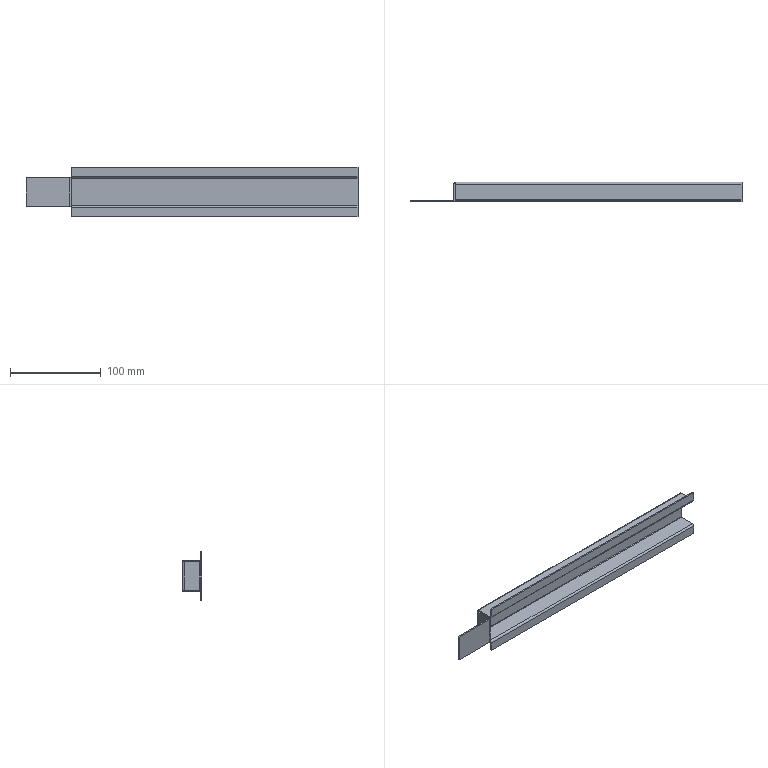Part | STEP file | 750078364 | 1 solid | 38 faces | box 366.5 x 21.5 x 55 mm | volume 47287 mm3 | plane 26 | cylinder 12 | commonest cylinder face diameters 1 x6 4 x6
STEP:
#1=CARTESIAN_POINT('',(-157.,20.,15.));
#2=VERTEX_POINT('',#1);
#3=CARTESIAN_POINT('',(-157.,20.,-15.));
#4=VERTEX_POINT('',#3);
#5=CARTESIAN_POINT('',(-157.,20.,15.));
#6=DIRECTION('',(0.,0.,-1.));
#7=VECTOR('',#6,1000.);
#8=LINE('',#5,#7);
#9=EDGE_CURVE('',#2,#4,#8,.T.);
#10=ORIENTED_EDGE('',*,*,#9,.F.);
#11=CARTESIAN_POINT('',(159.,20.,15.));
#12=VERTEX_POINT('',#11);
#13=CARTESIAN_POINT('',(159.,20.,15.));
#14=DIRECTION('',(-1.,0.,0.));
#15=VECTOR('',#14,1000.);
#16=LINE('',#13,#15);
#17=EDGE_CURVE('',#12,#2,#16,.T.);
#18=ORIENTED_EDGE('',*,*,#17,.F.);
#19=CARTESIAN_POINT('',(159.,20.,-15.));
#20=VERTEX_POINT('',#19);
#21=CARTESIAN_POINT('',(159.,20.,15.));
#22=DIRECTION('',(0.,0.,1.));
#23=VECTOR('',#22,1000.);
#24=LINE('',#21,#23);
#25=EDGE_CURVE('',#20,#12,#24,.T.);
#26=ORIENTED_EDGE('',*,*,#25,.F.);
#27=CARTESIAN_POINT('',(159.,20.,-15.));
#28=DIRECTION('',(1.,0.,0.));
#29=VECTOR('',#28,1000.);
#30=LINE('',#27,#29);
#31=EDGE_CURVE('',#4,#20,#30,.T.);
#32=ORIENTED_EDGE('',*,*,#31,.F.);
#33=EDGE_LOOP('',(#10,#18,#26,#32));
#34=FACE_OUTER_BOUND('',#33,.T.);
#35=CARTESIAN_POINT('',(159.,20.,15.));
#36=DIRECTION('',(0.,-1.,0.));
#37=DIRECTION('',(1.,0.,0.));
#38=AXIS2_PLACEMENT_3D('',#35,#36,#37);
#39=PLANE('',#38);
#40=ADVANCED_FACE('',(#34),#39,.F.);
#41=CARTESIAN_POINT('',(159.,18.,-17.));
#42=VERTEX_POINT('',#41);
#43=CARTESIAN_POINT('',(-157.498,18.,-17.));
#44=VERTEX_POINT('',#43);
#45=CARTESIAN_POINT('',(-157.,18.,-17.));
#46=DIRECTION('',(-1.,0.,0.));
#47=VECTOR('',#46,1000.);
#48=LINE('',#45,#47);
#49=EDGE_CURVE('',#42,#44,#48,.T.);
#50=ORIENTED_EDGE('',*,*,#49,.T.);
#51=CARTESIAN_POINT('',(-157.498,19.936,-15.5));
#52=VERTEX_POINT('',#51);
#53=CARTESIAN_POINT('',(-157.498,18.,-15.));
#54=DIRECTION('',(1.,0.,0.));
#55=DIRECTION('',(0.,1.,0.));
#56=AXIS2_PLACEMENT_3D('',#53,#54,#55);
#57=CIRCLE('',#56,2.);
#58=EDGE_CURVE('',#44,#52,#57,.T.);
#59=ORIENTED_EDGE('',*,*,#58,.T.);
#60=CARTESIAN_POINT('',(-157.,20.,-15.));
#61=CARTESIAN_POINT('',(-157.168,20.,-15.169));
#62=CARTESIAN_POINT('',(-157.335,19.979,-15.336));
#63=CARTESIAN_POINT('',(-157.498,19.936,-15.5));
#64=(BOUNDED_CURVE()B_SPLINE_CURVE(3,(#60,#61,#62,#63),.UNSPECIFIED.,.F.,.F.)B_SPLINE_CURVE_WITH_KNOTS((4,4),(1.571,1.823),.UNSPECIFIED.)CURVE()GEOMETRIC_REPRESENTATION_ITEM()RATIONAL_B_SPLINE_CURVE((1.,0.9947,0.9947,1.))REPRESENTATION_ITEM(''));
#65=EDGE_CURVE('',#4,#52,#64,.T.);
#66=ORIENTED_EDGE('',*,*,#65,.F.);
#67=ORIENTED_EDGE('',*,*,#31,.T.);
#68=CARTESIAN_POINT('',(159.,18.,-15.));
#69=DIRECTION('',(-1.,0.,0.));
#70=DIRECTION('',(0.,1.,0.));
#71=AXIS2_PLACEMENT_3D('',#68,#69,#70);
#72=CIRCLE('',#71,2.);
#73=EDGE_CURVE('',#20,#42,#72,.T.);
#74=ORIENTED_EDGE('',*,*,#73,.T.);
#75=EDGE_LOOP('',(#50,#59,#66,#67,#74));
#76=FACE_OUTER_BOUND('',#75,.T.);
#77=CARTESIAN_POINT('',(-157.,18.,-15.));
#78=DIRECTION('',(1.,0.,0.));
#79=DIRECTION('',(0.,1.,0.));
#80=AXIS2_PLACEMENT_3D('',#77,#78,#79);
#81=CYLINDRICAL_SURFACE('',#80,2.);
#82=ADVANCED_FACE('',(#76),#81,.T.);
#83=CARTESIAN_POINT('',(-159.,18.,-15.498));
#84=VERTEX_POINT('',#83);
#85=CARTESIAN_POINT('',(-159.,18.,15.498));
#86=VERTEX_POINT('',#85);
#87=CARTESIAN_POINT('',(-159.,18.,15.));
#88=DIRECTION('',(0.,0.,1.));
#89=VECTOR('',#88,1000.);
#90=LINE('',#87,#89);
#91=EDGE_CURVE('',#84,#86,#90,.T.);
#92=ORIENTED_EDGE('',*,*,#91,.T.);
#93=CARTESIAN_POINT('',(-157.5,19.936,15.498));
#94=VERTEX_POINT('',#93);
#95=CARTESIAN_POINT('',(-157.,18.,15.498));
#96=DIRECTION('',(0.,0.,-1.));
#97=DIRECTION('',(-1.,0.,0.));
#98=AXIS2_PLACEMENT_3D('',#95,#96,#97);
#99=CIRCLE('',#98,2.);
#100=EDGE_CURVE('',#86,#94,#99,.T.);
#101=ORIENTED_EDGE('',*,*,#100,.T.);
#102=CARTESIAN_POINT('',(-157.,20.,15.));
#103=CARTESIAN_POINT('',(-157.169,20.,15.168));
#104=CARTESIAN_POINT('',(-157.336,19.979,15.335));
#105=CARTESIAN_POINT('',(-157.5,19.936,15.498));
#106=(BOUNDED_CURVE()B_SPLINE_CURVE(3,(#102,#103,#104,#105),.UNSPECIFIED.,.F.,.F.)B_SPLINE_CURVE_WITH_KNOTS((4,4),(1.571,1.823),.UNSPECIFIED.)CURVE()GEOMETRIC_REPRESENTATION_ITEM()RATIONAL_B_SPLINE_CURVE((1.,0.9947,0.9947,1.))REPRESENTATION_ITEM(''));
#107=EDGE_CURVE('',#2,#94,#106,.T.);
#108=ORIENTED_EDGE('',*,*,#107,.F.);
#109=ORIENTED_EDGE('',*,*,#9,.T.);
#110=CARTESIAN_POINT('',(-157.5,19.936,-15.498));
#111=VERTEX_POINT('',#110);
#112=CARTESIAN_POINT('',(-157.,20.,-15.));
#113=CARTESIAN_POINT('',(-157.169,20.,-15.168));
#114=CARTESIAN_POINT('',(-157.336,19.979,-15.335));
#115=CARTESIAN_POINT('',(-157.5,19.936,-15.498));
#116=(BOUNDED_CURVE()B_SPLINE_CURVE(3,(#112,#113,#114,#115),.UNSPECIFIED.,.F.,.F.)B_SPLINE_CURVE_WITH_KNOTS((4,4),(4.712,4.965),.UNSPECIFIED.)CURVE()GEOMETRIC_REPRESENTATION_ITEM()RATIONAL_B_SPLINE_CURVE((1.,0.9947,0.9947,1.))REPRESENTATION_ITEM(''));
#117=EDGE_CURVE('',#4,#111,#116,.T.);
#118=ORIENTED_EDGE('',*,*,#117,.T.);
#119=CARTESIAN_POINT('',(-157.,18.,-15.498));
#120=DIRECTION('',(0.,0.,1.));
#121=DIRECTION('',(-1.,0.,0.));
#122=AXIS2_PLACEMENT_3D('',#119,#120,#121);
#123=CIRCLE('',#122,2.);
#124=EDGE_CURVE('',#111,#84,#123,.T.);
#125=ORIENTED_EDGE('',*,*,#124,.T.);
#126=EDGE_LOOP('',(#92,#101,#108,#109,#118,#125));
#127=FACE_OUTER_BOUND('',#126,.T.);
#128=CARTESIAN_POINT('',(-157.,18.,15.));
#129=DIRECTION('',(0.,0.,-1.));
#130=DIRECTION('',(-1.,0.,0.));
#131=AXIS2_PLACEMENT_3D('',#128,#129,#130);
#132=CYLINDRICAL_SURFACE('',#131,2.);
#133=ADVANCED_FACE('',(#127),#132,.T.);
#134=CARTESIAN_POINT('',(-157.498,18.,17.));
#135=VERTEX_POINT('',#134);
#136=CARTESIAN_POINT('',(159.,18.,17.));
#137=VERTEX_POINT('',#136);
#138=CARTESIAN_POINT('',(159.,18.,17.));
#139=DIRECTION('',(1.,0.,0.));
#140=VECTOR('',#139,1000.);
#141=LINE('',#138,#140);
#142=EDGE_CURVE('',#135,#137,#141,.T.);
#143=ORIENTED_EDGE('',*,*,#142,.T.);
#144=CARTESIAN_POINT('',(159.,18.,15.));
#145=DIRECTION('',(-1.,0.,0.));
#146=DIRECTION('',(0.,-1.,0.));
#147=AXIS2_PLACEMENT_3D('',#144,#145,#146);
#148=CIRCLE('',#147,2.);
#149=EDGE_CURVE('',#137,#12,#148,.T.);
#150=ORIENTED_EDGE('',*,*,#149,.T.);
#151=ORIENTED_EDGE('',*,*,#17,.T.);
#152=CARTESIAN_POINT('',(-157.498,19.936,15.5));
#153=VERTEX_POINT('',#152);
#154=CARTESIAN_POINT('',(-157.,20.,15.));
#155=CARTESIAN_POINT('',(-157.168,20.,15.169));
#156=CARTESIAN_POINT('',(-157.335,19.979,15.336));
#157=CARTESIAN_POINT('',(-157.498,19.936,15.5));
#158=(BOUNDED_CURVE()B_SPLINE_CURVE(3,(#154,#155,#156,#157),.UNSPECIFIED.,.F.,.F.)B_SPLINE_CURVE_WITH_KNOTS((4,4),(4.712,4.965),.UNSPECIFIED.)CURVE()GEOMETRIC_REPRESENTATION_ITEM()RATIONAL_B_SPLINE_CURVE((1.,0.9947,0.9947,1.))REPRESENTATION_ITEM(''));
#159=EDGE_CURVE('',#2,#153,#158,.T.);
#160=ORIENTED_EDGE('',*,*,#159,.T.);
#161=CARTESIAN_POINT('',(-157.498,18.,15.));
#162=DIRECTION('',(1.,0.,0.));
#163=DIRECTION('',(0.,-1.,0.));
#164=AXIS2_PLACEMENT_3D('',#161,#162,#163);
#165=CIRCLE('',#164,2.);
#166=EDGE_CURVE('',#153,#135,#165,.T.);
#167=ORIENTED_EDGE('',*,*,#166,.T.);
#168=EDGE_LOOP('',(#143,#150,#151,#160,#167));
#169=FACE_OUTER_BOUND('',#168,.T.);
#170=CARTESIAN_POINT('',(159.,18.,15.));
#171=DIRECTION('',(-1.,0.,0.));
#172=DIRECTION('',(0.,-1.,0.));
#173=AXIS2_PLACEMENT_3D('',#170,#171,#172);
#174=CYLINDRICAL_SURFACE('',#173,2.);
#175=ADVANCED_FACE('',(#169),#174,.T.);
#176=ORIENTED_EDGE('',*,*,#25,.T.);
#177=ORIENTED_EDGE('',*,*,#149,.F.);
#178=CARTESIAN_POINT('',(159.,0.5,17.));
#179=VERTEX_POINT('',#178);
#180=CARTESIAN_POINT('',(159.,20.,17.));
#181=DIRECTION('',(0.,1.,0.));
#182=VECTOR('',#181,1000.);
#183=LINE('',#180,#182);
#184=EDGE_CURVE('',#179,#137,#183,.T.);
#185=ORIENTED_EDGE('',*,*,#184,.F.);
#186=CARTESIAN_POINT('',(159.,0.,17.5));
#187=VERTEX_POINT('',#186);
#188=CARTESIAN_POINT('',(159.,0.5,17.5));
#189=DIRECTION('',(-1.,0.,0.));
#190=DIRECTION('',(0.,1.,0.));
#191=AXIS2_PLACEMENT_3D('',#188,#189,#190);
#192=CIRCLE('',#191,0.5);
#193=EDGE_CURVE('',#179,#187,#192,.T.);
#194=ORIENTED_EDGE('',*,*,#193,.T.);
#195=CARTESIAN_POINT('',(159.,0.,27.5));
#196=VERTEX_POINT('',#195);
#197=CARTESIAN_POINT('',(159.,0.,15.));
#198=DIRECTION('',(0.,0.,-1.));
#199=VECTOR('',#198,1000.);
#200=LINE('',#197,#199);
#201=EDGE_CURVE('',#196,#187,#200,.T.);
#202=ORIENTED_EDGE('',*,*,#201,.F.);
#203=CARTESIAN_POINT('',(159.,-1.5,27.5));
#204=VERTEX_POINT('',#203);
#205=CARTESIAN_POINT('',(159.,0.,27.5));
#206=DIRECTION('',(0.,1.,0.));
#207=VECTOR('',#206,1000.);
#208=LINE('',#205,#207);
#209=EDGE_CURVE('',#204,#196,#208,.T.);
#210=ORIENTED_EDGE('',*,*,#209,.F.);
#211=CARTESIAN_POINT('',(159.,-1.5,17.5));
#212=VERTEX_POINT('',#211);
#213=CARTESIAN_POINT('',(159.,-1.5,15.));
#214=DIRECTION('',(0.,0.,1.));
#215=VECTOR('',#214,1000.);
#216=LINE('',#213,#215);
#217=EDGE_CURVE('',#212,#204,#216,.T.);
#218=ORIENTED_EDGE('',*,*,#217,.F.);
#219=CARTESIAN_POINT('',(159.,0.5,15.5));
#220=VERTEX_POINT('',#219);
#221=CARTESIAN_POINT('',(159.,0.5,17.5));
#222=DIRECTION('',(-1.,0.,0.));
#223=DIRECTION('',(0.,1.,0.));
#224=AXIS2_PLACEMENT_3D('',#221,#222,#223);
#225=CIRCLE('',#224,2.);
#226=EDGE_CURVE('',#220,#212,#225,.T.);
#227=ORIENTED_EDGE('',*,*,#226,.F.);
#228=CARTESIAN_POINT('',(159.,18.,15.5));
#229=VERTEX_POINT('',#228);
#230=CARTESIAN_POINT('',(159.,20.,15.5));
#231=DIRECTION('',(0.,-1.,0.));
#232=VECTOR('',#231,1000.);
#233=LINE('',#230,#232);
#234=EDGE_CURVE('',#229,#220,#233,.T.);
#235=ORIENTED_EDGE('',*,*,#234,.F.);
#236=CARTESIAN_POINT('',(159.,18.5,15.));
#237=VERTEX_POINT('',#236);
#238=CARTESIAN_POINT('',(159.,18.,15.));
#239=DIRECTION('',(-1.,0.,0.));
#240=DIRECTION('',(0.,-1.,0.));
#241=AXIS2_PLACEMENT_3D('',#238,#239,#240);
#242=CIRCLE('',#241,0.5);
#243=EDGE_CURVE('',#229,#237,#242,.T.);
#244=ORIENTED_EDGE('',*,*,#243,.T.);
#245=CARTESIAN_POINT('',(159.,18.5,-15.));
#246=VERTEX_POINT('',#245);
#247=CARTESIAN_POINT('',(159.,18.5,15.));
#248=DIRECTION('',(0.,0.,1.));
#249=VECTOR('',#248,1000.);
#250=LINE('',#247,#249);
#251=EDGE_CURVE('',#246,#237,#250,.T.);
#252=ORIENTED_EDGE('',*,*,#251,.F.);
#253=CARTESIAN_POINT('',(159.,18.,-15.5));
#254=VERTEX_POINT('',#253);
#255=CARTESIAN_POINT('',(159.,18.,-15.));
#256=DIRECTION('',(-1.,0.,0.));
#257=DIRECTION('',(0.,1.,0.));
#258=AXIS2_PLACEMENT_3D('',#255,#256,#257);
#259=CIRCLE('',#258,0.5);
#260=EDGE_CURVE('',#246,#254,#259,.T.);
#261=ORIENTED_EDGE('',*,*,#260,.T.);
#262=CARTESIAN_POINT('',(159.,0.5,-15.5));
#263=VERTEX_POINT('',#262);
#264=CARTESIAN_POINT('',(159.,20.,-15.5));
#265=DIRECTION('',(0.,1.,0.));
#266=VECTOR('',#265,1000.);
#267=LINE('',#264,#266);
#268=EDGE_CURVE('',#263,#254,#267,.T.);
#269=ORIENTED_EDGE('',*,*,#268,.F.);
#270=CARTESIAN_POINT('',(159.,-1.5,-17.5));
#271=VERTEX_POINT('',#270);
#272=CARTESIAN_POINT('',(159.,0.5,-17.5));
#273=DIRECTION('',(-1.,0.,0.));
#274=DIRECTION('',(0.,-1.,0.));
#275=AXIS2_PLACEMENT_3D('',#272,#273,#274);
#276=CIRCLE('',#275,2.);
#277=EDGE_CURVE('',#271,#263,#276,.T.);
#278=ORIENTED_EDGE('',*,*,#277,.F.);
#279=CARTESIAN_POINT('',(159.,-1.5,-27.5));
#280=VERTEX_POINT('',#279);
#281=CARTESIAN_POINT('',(159.,-1.5,15.));
#282=DIRECTION('',(0.,0.,1.));
#283=VECTOR('',#282,1000.);
#284=LINE('',#281,#283);
#285=EDGE_CURVE('',#280,#271,#284,.T.);
#286=ORIENTED_EDGE('',*,*,#285,.F.);
#287=CARTESIAN_POINT('',(159.,0.,-27.5));
#288=VERTEX_POINT('',#287);
#289=CARTESIAN_POINT('',(159.,0.,-27.5));
#290=DIRECTION('',(0.,-1.,0.));
#291=VECTOR('',#290,1000.);
#292=LINE('',#289,#291);
#293=EDGE_CURVE('',#288,#280,#292,.T.);
#294=ORIENTED_EDGE('',*,*,#293,.F.);
#295=CARTESIAN_POINT('',(159.,0.,-17.5));
#296=VERTEX_POINT('',#295);
#297=CARTESIAN_POINT('',(159.,0.,15.));
#298=DIRECTION('',(0.,0.,-1.));
#299=VECTOR('',#298,1000.);
#300=LINE('',#297,#299);
#301=EDGE_CURVE('',#296,#288,#300,.T.);
#302=ORIENTED_EDGE('',*,*,#301,.F.);
#303=CARTESIAN_POINT('',(159.,0.5,-17.));
#304=VERTEX_POINT('',#303);
#305=CARTESIAN_POINT('',(159.,0.5,-17.5));
#306=DIRECTION('',(1.,0.,0.));
#307=DIRECTION('',(0.,-1.,0.));
#308=AXIS2_PLACEMENT_3D('',#305,#306,#307);
#309=CIRCLE('',#308,0.5);
#310=EDGE_CURVE('',#304,#296,#309,.T.);
#311=ORIENTED_EDGE('',*,*,#310,.F.);
#312=CARTESIAN_POINT('',(159.,18.,-17.));
#313=DIRECTION('',(0.,1.,0.));
#314=VECTOR('',#313,1000.);
#315=LINE('',#312,#314);
#316=EDGE_CURVE('',#304,#42,#315,.T.);
#317=ORIENTED_EDGE('',*,*,#316,.T.);
#318=ORIENTED_EDGE('',*,*,#73,.F.);
#319=EDGE_LOOP('',(#176,#177,#185,#194,#202,#210,#218,#227,#235,#244,#252,#261,#269,#278,#286,#294,#302,#311,#317,#318));
#320=FACE_OUTER_BOUND('',#319,.T.);
#321=CARTESIAN_POINT('',(159.,20.,15.));
#322=DIRECTION('',(-1.,0.,0.));
#323=DIRECTION('',(0.,-1.,0.));
#324=AXIS2_PLACEMENT_3D('',#321,#322,#323);
#325=PLANE('',#324);
#326=ADVANCED_FACE('',(#320),#325,.F.);
#327=CARTESIAN_POINT('',(-157.498,-1.5,-27.5));
#328=VERTEX_POINT('',#327);
#329=CARTESIAN_POINT('',(-157.498,-1.5,-17.5));
#330=VERTEX_POINT('',#329);
#331=CARTESIAN_POINT('',(-157.498,-1.5,-15.5));
#332=DIRECTION('',(0.,0.,1.));
#333=VECTOR('',#332,1000.);
#334=LINE('',#331,#333);
#335=EDGE_CURVE('',#328,#330,#334,.T.);
#336=ORIENTED_EDGE('',*,*,#335,.T.);
#337=CARTESIAN_POINT('',(-157.498,0.5,-15.5));
#338=VERTEX_POINT('',#337);
#339=CARTESIAN_POINT('',(-157.498,0.5,-17.5));
#340=DIRECTION('',(-1.,0.,0.));
#341=DIRECTION('',(0.,-1.,0.));
#342=AXIS2_PLACEMENT_3D('',#339,#340,#341);
#343=CIRCLE('',#342,2.);
#344=EDGE_CURVE('',#330,#338,#343,.T.);
#345=ORIENTED_EDGE('',*,*,#344,.T.);
#346=CARTESIAN_POINT('',(-157.498,18.,-15.5));
#347=VERTEX_POINT('',#346);
#348=CARTESIAN_POINT('',(-157.498,18.,-15.5));
#349=DIRECTION('',(0.,1.,0.));
#350=VECTOR('',#349,1000.);
#351=LINE('',#348,#350);
#352=EDGE_CURVE('',#338,#347,#351,.T.);
#353=ORIENTED_EDGE('',*,*,#352,.T.);
#354=CARTESIAN_POINT('',(-157.498,18.,-15.5));
#355=DIRECTION('',(0.,1.,0.));
#356=VECTOR('',#355,1000.);
#357=LINE('',#354,#356);
#358=EDGE_CURVE('',#347,#52,#357,.T.);
#359=ORIENTED_EDGE('',*,*,#358,.T.);
#360=ORIENTED_EDGE('',*,*,#58,.F.);
#361=CARTESIAN_POINT('',(-157.498,0.5,-17.));
#362=VERTEX_POINT('',#361);
#363=CARTESIAN_POINT('',(-157.498,18.,-17.));
#364=DIRECTION('',(0.,-1.,0.));
#365=VECTOR('',#364,1000.);
#366=LINE('',#363,#365);
#367=EDGE_CURVE('',#44,#362,#366,.T.);
#368=ORIENTED_EDGE('',*,*,#367,.T.);
#369=CARTESIAN_POINT('',(-157.498,0.,-17.5));
#370=VERTEX_POINT('',#369);
#371=CARTESIAN_POINT('',(-157.498,0.5,-17.5));
#372=DIRECTION('',(1.,0.,0.));
#373=DIRECTION('',(0.,-1.,0.));
#374=AXIS2_PLACEMENT_3D('',#371,#372,#373);
#375=CIRCLE('',#374,0.5);
#376=EDGE_CURVE('',#362,#370,#375,.T.);
#377=ORIENTED_EDGE('',*,*,#376,.T.);
#378=CARTESIAN_POINT('',(-157.498,0.,-27.5));
#379=VERTEX_POINT('',#378);
#380=CARTESIAN_POINT('',(-157.498,0.,-15.5));
#381=DIRECTION('',(0.,0.,-1.));
#382=VECTOR('',#381,1000.);
#383=LINE('',#380,#382);
#384=EDGE_CURVE('',#370,#379,#383,.T.);
#385=ORIENTED_EDGE('',*,*,#384,.T.);
#386=CARTESIAN_POINT('',(-157.498,0.,-27.5));
#387=DIRECTION('',(0.,1.,0.));
#388=VECTOR('',#387,1000.);
#389=LINE('',#386,#388);
#390=EDGE_CURVE('',#328,#379,#389,.T.);
#391=ORIENTED_EDGE('',*,*,#390,.F.);
#392=EDGE_LOOP('',(#336,#345,#353,#359,#360,#368,#377,#385,#391));
#393=FACE_OUTER_BOUND('',#392,.T.);
#394=CARTESIAN_POINT('',(-157.498,18.,-15.5));
#395=DIRECTION('',(-1.,0.,0.));
#396=DIRECTION('',(0.,0.,1.));
#397=AXIS2_PLACEMENT_3D('',#394,#395,#396);
#398=PLANE('',#397);
#399=ADVANCED_FACE('',(#393),#398,.T.);
#400=CARTESIAN_POINT('',(-157.,0.5,-17.));
#401=DIRECTION('',(1.,0.,0.));
#402=VECTOR('',#401,1000.);
#403=LINE('',#400,#402);
#404=EDGE_CURVE('',#362,#304,#403,.T.);
#405=ORIENTED_EDGE('',*,*,#404,.F.);
#406=ORIENTED_EDGE('',*,*,#367,.F.);
#407=ORIENTED_EDGE('',*,*,#49,.F.);
#408=ORIENTED_EDGE('',*,*,#316,.F.);
#409=EDGE_LOOP('',(#405,#406,#407,#408));
#410=FACE_OUTER_BOUND('',#409,.T.);
#411=CARTESIAN_POINT('',(-157.,18.,-17.));
#412=DIRECTION('',(0.,0.,1.));
#413=DIRECTION('',(0.,-1.,0.));
#414=AXIS2_PLACEMENT_3D('',#411,#412,#413);
#415=PLANE('',#414);
#416=ADVANCED_FACE('',(#410),#415,.F.);
#417=CARTESIAN_POINT('',(-207.5,-1.5,15.498));
#418=VERTEX_POINT('',#417);
#419=CARTESIAN_POINT('',(-159.5,-1.5,15.498));
#420=VERTEX_POINT('',#419);
#421=CARTESIAN_POINT('',(-159.,-1.5,15.498));
#422=DIRECTION('',(1.,0.,0.));
#423=VECTOR('',#422,1000.);
#424=LINE('',#421,#423);
#425=EDGE_CURVE('',#418,#420,#424,.T.);
#426=ORIENTED_EDGE('',*,*,#425,.T.);
#427=CARTESIAN_POINT('',(-157.5,0.5,15.498));
#428=VERTEX_POINT('',#427);
#429=CARTESIAN_POINT('',(-159.5,0.5,15.498));
#430=DIRECTION('',(0.,0.,1.));
#431=DIRECTION('',(-1.,0.,0.));
#432=AXIS2_PLACEMENT_3D('',#429,#430,#431);
#433=CIRCLE('',#432,2.);
#434=EDGE_CURVE('',#420,#428,#433,.T.);
#435=ORIENTED_EDGE('',*,*,#434,.T.);
#436=CARTESIAN_POINT('',(-157.5,18.,15.498));
#437=VERTEX_POINT('',#436);
#438=CARTESIAN_POINT('',(-157.5,0.,15.498));
#439=DIRECTION('',(0.,1.,0.));
#440=VECTOR('',#439,1000.);
#441=LINE('',#438,#440);
#442=EDGE_CURVE('',#428,#437,#441,.T.);
#443=ORIENTED_EDGE('',*,*,#442,.T.);
#444=CARTESIAN_POINT('',(-157.5,0.,15.498));
#445=DIRECTION('',(0.,1.,0.));
#446=VECTOR('',#445,1000.);
#447=LINE('',#444,#446);
#448=EDGE_CURVE('',#437,#94,#447,.T.);
#449=ORIENTED_EDGE('',*,*,#448,.T.);
#450=ORIENTED_EDGE('',*,*,#100,.F.);
#451=CARTESIAN_POINT('',(-159.,0.5,15.498));
#452=VERTEX_POINT('',#451);
#453=CARTESIAN_POINT('',(-159.,0.,15.498));
#454=DIRECTION('',(0.,-1.,0.));
#455=VECTOR('',#454,1000.);
#456=LINE('',#453,#455);
#457=EDGE_CURVE('',#86,#452,#456,.T.);
#458=ORIENTED_EDGE('',*,*,#457,.T.);
#459=CARTESIAN_POINT('',(-159.5,0.,15.498));
#460=VERTEX_POINT('',#459);
#461=CARTESIAN_POINT('',(-159.5,0.5,15.498));
#462=DIRECTION('',(0.,0.,-1.));
#463=DIRECTION('',(-1.,0.,0.));
#464=AXIS2_PLACEMENT_3D('',#461,#462,#463);
#465=CIRCLE('',#464,0.5);
#466=EDGE_CURVE('',#452,#460,#465,.T.);
#467=ORIENTED_EDGE('',*,*,#466,.T.);
#468=CARTESIAN_POINT('',(-207.5,0.,15.498));
#469=VERTEX_POINT('',#468);
#470=CARTESIAN_POINT('',(-159.,0.,15.498));
#471=DIRECTION('',(-1.,0.,0.));
#472=VECTOR('',#471,1000.);
#473=LINE('',#470,#472);
#474=EDGE_CURVE('',#460,#469,#473,.T.);
#475=ORIENTED_EDGE('',*,*,#474,.T.);
#476=CARTESIAN_POINT('',(-207.5,0.,15.498));
#477=DIRECTION('',(0.,1.,0.));
#478=VECTOR('',#477,1000.);
#479=LINE('',#476,#478);
#480=EDGE_CURVE('',#418,#469,#479,.T.);
#481=ORIENTED_EDGE('',*,*,#480,.F.);
#482=EDGE_LOOP('',(#426,#435,#443,#449,#450,#458,#467,#475,#481));
#483=FACE_OUTER_BOUND('',#482,.T.);
#484=CARTESIAN_POINT('',(-159.,0.,15.498));
#485=DIRECTION('',(0.,0.,1.));
#486=DIRECTION('',(1.,0.,0.));
#487=AXIS2_PLACEMENT_3D('',#484,#485,#486);
#488=PLANE('',#487);
#489=ADVANCED_FACE('',(#483),#488,.T.);
#490=CARTESIAN_POINT('',(-159.,0.5,-15.498));
#491=VERTEX_POINT('',#490);
#492=CARTESIAN_POINT('',(-159.,0.5,15.));
#493=DIRECTION('',(0.,0.,-1.));
#494=VECTOR('',#493,1000.);
#495=LINE('',#492,#494);
#496=EDGE_CURVE('',#452,#491,#495,.T.);
#497=ORIENTED_EDGE('',*,*,#496,.F.);
#498=ORIENTED_EDGE('',*,*,#457,.F.);
#499=ORIENTED_EDGE('',*,*,#91,.F.);
#500=CARTESIAN_POINT('',(-159.,20.,-15.498));
#501=DIRECTION('',(0.,1.,0.));
#502=VECTOR('',#501,1000.);
#503=LINE('',#500,#502);
#504=EDGE_CURVE('',#491,#84,#503,.T.);
#505=ORIENTED_EDGE('',*,*,#504,.F.);
#506=EDGE_LOOP('',(#497,#498,#499,#505));
#507=FACE_OUTER_BOUND('',#506,.T.);
#508=CARTESIAN_POINT('',(-159.,20.,15.));
#509=DIRECTION('',(1.,0.,0.));
#510=DIRECTION('',(0.,0.,-1.));
#511=AXIS2_PLACEMENT_3D('',#508,#509,#510);
#512=PLANE('',#511);
#513=ADVANCED_FACE('',(#507),#512,.F.);
#514=ORIENTED_EDGE('',*,*,#124,.F.);
#515=CARTESIAN_POINT('',(-157.5,18.,-15.498));
#516=VERTEX_POINT('',#515);
#517=CARTESIAN_POINT('',(-157.5,20.,-15.498));
#518=DIRECTION('',(0.,1.,0.));
#519=VECTOR('',#518,1000.);
#520=LINE('',#517,#519);
#521=EDGE_CURVE('',#516,#111,#520,.T.);
#522=ORIENTED_EDGE('',*,*,#521,.F.);
#523=CARTESIAN_POINT('',(-157.5,0.5,-15.498));
#524=VERTEX_POINT('',#523);
#525=CARTESIAN_POINT('',(-157.5,20.,-15.498));
#526=DIRECTION('',(0.,1.,0.));
#527=VECTOR('',#526,1000.);
#528=LINE('',#525,#527);
#529=EDGE_CURVE('',#524,#516,#528,.T.);
#530=ORIENTED_EDGE('',*,*,#529,.F.);
#531=CARTESIAN_POINT('',(-159.5,-1.5,-15.498));
#532=VERTEX_POINT('',#531);
#533=CARTESIAN_POINT('',(-159.5,0.5,-15.498));
#534=DIRECTION('',(0.,0.,1.));
#535=DIRECTION('',(-1.,0.,0.));
#536=AXIS2_PLACEMENT_3D('',#533,#534,#535);
#537=CIRCLE('',#536,2.);
#538=EDGE_CURVE('',#532,#524,#537,.T.);
#539=ORIENTED_EDGE('',*,*,#538,.F.);
#540=CARTESIAN_POINT('',(-207.5,-1.5,-15.498));
#541=VERTEX_POINT('',#540);
#542=CARTESIAN_POINT('',(159.,-1.5,-15.498));
#543=DIRECTION('',(1.,0.,0.));
#544=VECTOR('',#543,1000.);
#545=LINE('',#542,#544);
#546=EDGE_CURVE('',#541,#532,#545,.T.);
#547=ORIENTED_EDGE('',*,*,#546,.F.);
#548=CARTESIAN_POINT('',(-207.5,0.,-15.498));
#549=VERTEX_POINT('',#548);
#550=CARTESIAN_POINT('',(-207.5,0.,-15.498));
#551=DIRECTION('',(0.,-1.,0.));
#552=VECTOR('',#551,1000.);
#553=LINE('',#550,#552);
#554=EDGE_CURVE('',#549,#541,#553,.T.);
#555=ORIENTED_EDGE('',*,*,#554,.F.);
#556=CARTESIAN_POINT('',(-159.5,0.,-15.498));
#557=VERTEX_POINT('',#556);
#558=CARTESIAN_POINT('',(159.,0.,-15.498));
#559=DIRECTION('',(-1.,0.,0.));
#560=VECTOR('',#559,1000.);
#561=LINE('',#558,#560);
#562=EDGE_CURVE('',#557,#549,#561,.T.);
#563=ORIENTED_EDGE('',*,*,#562,.F.);
#564=CARTESIAN_POINT('',(-159.5,0.5,-15.498));
#565=DIRECTION('',(0.,0.,-1.));
#566=DIRECTION('',(-1.,0.,0.));
#567=AXIS2_PLACEMENT_3D('',#564,#565,#566);
#568=CIRCLE('',#567,0.5);
#569=EDGE_CURVE('',#491,#557,#568,.T.);
#570=ORIENTED_EDGE('',*,*,#569,.F.);
#571=ORIENTED_EDGE('',*,*,#504,.T.);
#572=EDGE_LOOP('',(#514,#522,#530,#539,#547,#555,#563,#570,#571));
#573=FACE_OUTER_BOUND('',#572,.T.);
#574=CARTESIAN_POINT('',(159.,20.,-15.498));
#575=DIRECTION('',(0.,0.,1.));
#576=DIRECTION('',(1.,0.,0.));
#577=AXIS2_PLACEMENT_3D('',#574,#575,#576);
#578=PLANE('',#577);
#579=ADVANCED_FACE('',(#573),#578,.F.);
#580=CARTESIAN_POINT('',(-157.498,0.5,17.));
#581=VERTEX_POINT('',#580);
#582=CARTESIAN_POINT('',(159.,0.5,17.));
#583=DIRECTION('',(-1.,0.,0.));
#584=VECTOR('',#583,1000.);
#585=LINE('',#582,#584);
#586=EDGE_CURVE('',#179,#581,#585,.T.);
#587=ORIENTED_EDGE('',*,*,#586,.F.);
#588=ORIENTED_EDGE('',*,*,#184,.T.);
#589=ORIENTED_EDGE('',*,*,#142,.F.);
#590=CARTESIAN_POINT('',(-157.498,18.,17.));
#591=DIRECTION('',(0.,1.,0.));
#592=VECTOR('',#591,1000.);
#593=LINE('',#590,#592);
#594=EDGE_CURVE('',#581,#135,#593,.T.);
#595=ORIENTED_EDGE('',*,*,#594,.F.);
#596=EDGE_LOOP('',(#587,#588,#589,#595));
#597=FACE_OUTER_BOUND('',#596,.T.);
#598=CARTESIAN_POINT('',(159.,18.,17.));
#599=DIRECTION('',(0.,0.,-1.));
#600=DIRECTION('',(-1.,0.,0.));
#601=AXIS2_PLACEMENT_3D('',#598,#599,#600);
#602=PLANE('',#601);
#603=ADVANCED_FACE('',(#597),#602,.F.);
#604=CARTESIAN_POINT('',(-157.498,0.,27.5));
#605=VERTEX_POINT('',#604);
#606=CARTESIAN_POINT('',(-157.498,0.,17.5));
#607=VERTEX_POINT('',#606);
#608=CARTESIAN_POINT('',(-157.498,0.,15.));
#609=DIRECTION('',(0.,0.,-1.));
#610=VECTOR('',#609,1000.);
#611=LINE('',#608,#610);
#612=EDGE_CURVE('',#605,#607,#611,.T.);
#613=ORIENTED_EDGE('',*,*,#612,.T.);
#614=CARTESIAN_POINT('',(-157.498,0.5,17.5));
#615=DIRECTION('',(1.,0.,0.));
#616=DIRECTION('',(0.,1.,0.));
#617=AXIS2_PLACEMENT_3D('',#614,#615,#616);
#618=CIRCLE('',#617,0.5);
#619=EDGE_CURVE('',#607,#581,#618,.T.);
#620=ORIENTED_EDGE('',*,*,#619,.T.);
#621=ORIENTED_EDGE('',*,*,#594,.T.);
#622=ORIENTED_EDGE('',*,*,#166,.F.);
#623=CARTESIAN_POINT('',(-157.498,18.,15.5));
#624=VERTEX_POINT('',#623);
#625=CARTESIAN_POINT('',(-157.498,18.,15.5));
#626=DIRECTION('',(0.,-1.,0.));
#627=VECTOR('',#626,1000.);
#628=LINE('',#625,#627);
#629=EDGE_CURVE('',#153,#624,#628,.T.);
#630=ORIENTED_EDGE('',*,*,#629,.T.);
#631=CARTESIAN_POINT('',(-157.498,0.5,15.5));
#632=VERTEX_POINT('',#631);
#633=CARTESIAN_POINT('',(-157.498,18.,15.5));
#634=DIRECTION('',(0.,-1.,0.));
#635=VECTOR('',#634,1000.);
#636=LINE('',#633,#635);
#637=EDGE_CURVE('',#624,#632,#636,.T.);
#638=ORIENTED_EDGE('',*,*,#637,.T.);
#639=CARTESIAN_POINT('',(-157.498,-1.5,17.5));
#640=VERTEX_POINT('',#639);
#641=CARTESIAN_POINT('',(-157.498,0.5,17.5));
#642=DIRECTION('',(-1.,0.,0.));
#643=DIRECTION('',(0.,1.,0.));
#644=AXIS2_PLACEMENT_3D('',#641,#642,#643);
#645=CIRCLE('',#644,2.);
#646=EDGE_CURVE('',#632,#640,#645,.T.);
#647=ORIENTED_EDGE('',*,*,#646,.T.);
#648=CARTESIAN_POINT('',(-157.498,-1.5,27.5));
#649=VERTEX_POINT('',#648);
#650=CARTESIAN_POINT('',(-157.498,-1.5,15.));
#651=DIRECTION('',(0.,0.,1.));
#652=VECTOR('',#651,1000.);
#653=LINE('',#650,#652);
#654=EDGE_CURVE('',#640,#649,#653,.T.);
#655=ORIENTED_EDGE('',*,*,#654,.T.);
#656=CARTESIAN_POINT('',(-157.498,0.,27.5));
#657=DIRECTION('',(0.,-1.,0.));
#658=VECTOR('',#657,1000.);
#659=LINE('',#656,#658);
#660=EDGE_CURVE('',#605,#649,#659,.T.);
#661=ORIENTED_EDGE('',*,*,#660,.F.);
#662=EDGE_LOOP('',(#613,#620,#621,#622,#630,#638,#647,#655,#661));
#663=FACE_OUTER_BOUND('',#662,.T.);
#664=CARTESIAN_POINT('',(-157.498,18.,15.));
#665=DIRECTION('',(-1.,0.,0.));
#666=DIRECTION('',(0.,-1.,0.));
#667=AXIS2_PLACEMENT_3D('',#664,#665,#666);
#668=PLANE('',#667);
#669=ADVANCED_FACE('',(#663),#668,.T.);
#670=CARTESIAN_POINT('',(-157.,18.5,15.));
#671=VERTEX_POINT('',#670);
#672=CARTESIAN_POINT('',(159.,18.5,15.));
#673=DIRECTION('',(-1.,0.,0.));
#674=VECTOR('',#673,1000.);
#675=LINE('',#672,#674);
#676=EDGE_CURVE('',#237,#671,#675,.T.);
#677=ORIENTED_EDGE('',*,*,#676,.T.);
#678=CARTESIAN_POINT('',(-157.,18.5,-15.));
#679=VERTEX_POINT('',#678);
#680=CARTESIAN_POINT('',(-157.,18.5,15.));
#681=DIRECTION('',(0.,0.,-1.));
#682=VECTOR('',#681,1000.);
#683=LINE('',#680,#682);
#684=EDGE_CURVE('',#671,#679,#683,.T.);
#685=ORIENTED_EDGE('',*,*,#684,.T.);
#686=CARTESIAN_POINT('',(159.,18.5,-15.));
#687=DIRECTION('',(1.,0.,0.));
#688=VECTOR('',#687,1000.);
#689=LINE('',#686,#688);
#690=EDGE_CURVE('',#679,#246,#689,.T.);
#691=ORIENTED_EDGE('',*,*,#690,.T.);
#692=ORIENTED_EDGE('',*,*,#251,.T.);
#693=EDGE_LOOP('',(#677,#685,#691,#692));
#694=FACE_OUTER_BOUND('',#693,.T.);
#695=CARTESIAN_POINT('',(159.,18.5,15.));
#696=DIRECTION('',(0.,-1.,0.));
#697=DIRECTION('',(1.,0.,0.));
#698=AXIS2_PLACEMENT_3D('',#695,#696,#697);
#699=PLANE('',#698);
#700=ADVANCED_FACE('',(#694),#699,.T.);
#701=ORIENTED_EDGE('',*,*,#277,.T.);
#702=CARTESIAN_POINT('',(159.,0.5,-15.5));
#703=DIRECTION('',(-1.,0.,0.));
#704=VECTOR('',#703,1000.);
#705=LINE('',#702,#704);
#706=EDGE_CURVE('',#263,#338,#705,.T.);
#707=ORIENTED_EDGE('',*,*,#706,.T.);
#708=ORIENTED_EDGE('',*,*,#344,.F.);
#709=CARTESIAN_POINT('',(159.,-1.5,-17.5));
#710=DIRECTION('',(1.,0.,0.));
#711=VECTOR('',#710,1000.);
#712=LINE('',#709,#711);
#713=EDGE_CURVE('',#330,#271,#712,.T.);
#714=ORIENTED_EDGE('',*,*,#713,.T.);
#715=EDGE_LOOP('',(#701,#707,#708,#714));
#716=FACE_OUTER_BOUND('',#715,.T.);
#717=CARTESIAN_POINT('',(159.,0.5,-17.5));
#718=DIRECTION('',(-1.,0.,0.));
#719=DIRECTION('',(0.,-1.,0.));
#720=AXIS2_PLACEMENT_3D('',#717,#718,#719);
#721=CYLINDRICAL_SURFACE('',#720,2.);
#722=ADVANCED_FACE('',(#716),#721,.T.);
#723=CARTESIAN_POINT('',(159.,-1.5,-27.5));
#724=DIRECTION('',(-1.,0.,0.));
#725=VECTOR('',#724,1000.);
#726=LINE('',#723,#725);
#727=EDGE_CURVE('',#280,#328,#726,.T.);
#728=ORIENTED_EDGE('',*,*,#727,.F.);
#729=ORIENTED_EDGE('',*,*,#285,.T.);
#730=ORIENTED_EDGE('',*,*,#713,.F.);
#731=ORIENTED_EDGE('',*,*,#335,.F.);
#732=EDGE_LOOP('',(#728,#729,#730,#731));
#733=FACE_OUTER_BOUND('',#732,.T.);
#734=CARTESIAN_POINT('',(159.,-1.5,-17.5));
#735=DIRECTION('',(0.,1.,0.));
#736=DIRECTION('',(0.,0.,1.));
#737=AXIS2_PLACEMENT_3D('',#734,#735,#736);
#738=PLANE('',#737);
#739=ADVANCED_FACE('',(#733),#738,.F.);
#740=ORIENTED_EDGE('',*,*,#301,.T.);
#741=CARTESIAN_POINT('',(159.,0.,-27.5));
#742=DIRECTION('',(-1.,0.,0.));
#743=VECTOR('',#742,1000.);
#744=LINE('',#741,#743);
#745=EDGE_CURVE('',#288,#379,#744,.T.);
#746=ORIENTED_EDGE('',*,*,#745,.T.);
#747=ORIENTED_EDGE('',*,*,#384,.F.);
#748=CARTESIAN_POINT('',(159.,0.,-17.5));
#749=DIRECTION('',(1.,0.,0.));
#750=VECTOR('',#749,1000.);
#751=LINE('',#748,#750);
#752=EDGE_CURVE('',#370,#296,#751,.T.);
#753=ORIENTED_EDGE('',*,*,#752,.T.);
#754=EDGE_LOOP('',(#740,#746,#747,#753));
#755=FACE_OUTER_BOUND('',#754,.T.);
#756=CARTESIAN_POINT('',(159.,0.,-17.5));
#757=DIRECTION('',(0.,1.,0.));
#758=DIRECTION('',(0.,0.,1.));
#759=AXIS2_PLACEMENT_3D('',#756,#757,#758);
#760=PLANE('',#759);
#761=ADVANCED_FACE('',(#755),#760,.T.);
#762=ORIENTED_EDGE('',*,*,#65,.T.);
#763=ORIENTED_EDGE('',*,*,#358,.F.);
#764=CARTESIAN_POINT('',(-157.498,18.,-15.5));
#765=CARTESIAN_POINT('',(-157.498,18.293,-15.5));
#766=CARTESIAN_POINT('',(-157.292,18.5,-15.293));
#767=CARTESIAN_POINT('',(-157.,18.5,-15.));
#768=(BOUNDED_CURVE()B_SPLINE_CURVE(3,(#764,#765,#766,#767),.UNSPECIFIED.,.F.,.F.)B_SPLINE_CURVE_WITH_KNOTS((4,4),(3.142,4.712),.UNSPECIFIED.)CURVE()GEOMETRIC_REPRESENTATION_ITEM()RATIONAL_B_SPLINE_CURVE((1.,0.8047,0.8047,1.))REPRESENTATION_ITEM(''));
#769=EDGE_CURVE('',#347,#679,#768,.T.);
#770=ORIENTED_EDGE('',*,*,#769,.T.);
#771=CARTESIAN_POINT('',(-157.,1020.,-15.));
#772=DIRECTION('',(0.,1.,0.));
#773=VECTOR('',#772,1000.);
#774=LINE('',#771,#773);
#775=EDGE_CURVE('',#679,#4,#774,.T.);
#776=ORIENTED_EDGE('',*,*,#775,.T.);
#777=EDGE_LOOP('',(#762,#763,#770,#776));
#778=FACE_OUTER_BOUND('',#777,.T.);
#779=CARTESIAN_POINT('',(548.688,1020.,693.522));
#780=DIRECTION('',(-0.7085,0.,0.7057));
#781=DIRECTION('',(0.7057,0.,0.7085));
#782=AXIS2_PLACEMENT_3D('',#779,#780,#781);
#783=PLANE('',#782);
#784=ADVANCED_FACE('',(#778),#783,.T.);
#785=ORIENTED_EDGE('',*,*,#352,.F.);
#786=ORIENTED_EDGE('',*,*,#706,.F.);
#787=ORIENTED_EDGE('',*,*,#268,.T.);
#788=CARTESIAN_POINT('',(-157.,18.,-15.5));
#789=DIRECTION('',(-1.,0.,0.));
#790=VECTOR('',#789,1000.);
#791=LINE('',#788,#790);
#792=EDGE_CURVE('',#254,#347,#791,.T.);
#793=ORIENTED_EDGE('',*,*,#792,.T.);
#794=EDGE_LOOP('',(#785,#786,#787,#793));
#795=FACE_OUTER_BOUND('',#794,.T.);
#796=CARTESIAN_POINT('',(-157.,18.,-15.5));
#797=DIRECTION('',(0.,0.,1.));
#798=DIRECTION('',(0.,-1.,0.));
#799=AXIS2_PLACEMENT_3D('',#796,#797,#798);
#800=PLANE('',#799);
#801=ADVANCED_FACE('',(#795),#800,.T.);
#802=ORIENTED_EDGE('',*,*,#404,.T.);
#803=ORIENTED_EDGE('',*,*,#310,.T.);
#804=ORIENTED_EDGE('',*,*,#752,.F.);
#805=ORIENTED_EDGE('',*,*,#376,.F.);
#806=EDGE_LOOP('',(#802,#803,#804,#805));
#807=FACE_OUTER_BOUND('',#806,.T.);
#808=CARTESIAN_POINT('',(159.,0.5,-17.5));
#809=DIRECTION('',(-1.,0.,0.));
#810=DIRECTION('',(0.,-1.,0.));
#811=AXIS2_PLACEMENT_3D('',#808,#809,#810);
#812=CYLINDRICAL_SURFACE('',#811,0.5);
#813=ADVANCED_FACE('',(#807),#812,.F.);
#814=ORIENTED_EDGE('',*,*,#434,.F.);
#815=CARTESIAN_POINT('',(-159.5,-1.5,15.));
#816=DIRECTION('',(0.,0.,-1.));
#817=VECTOR('',#816,1000.);
#818=LINE('',#815,#817);
#819=EDGE_CURVE('',#420,#532,#818,.T.);
#820=ORIENTED_EDGE('',*,*,#819,.T.);
#821=ORIENTED_EDGE('',*,*,#538,.T.);
#822=CARTESIAN_POINT('',(-157.5,0.5,15.));
#823=DIRECTION('',(0.,0.,1.));
#824=VECTOR('',#823,1000.);
#825=LINE('',#822,#824);
#826=EDGE_CURVE('',#524,#428,#825,.T.);
#827=ORIENTED_EDGE('',*,*,#826,.T.);
#828=EDGE_LOOP('',(#814,#820,#821,#827));
#829=FACE_OUTER_BOUND('',#828,.T.);
#830=CARTESIAN_POINT('',(-159.5,0.5,15.));
#831=DIRECTION('',(0.,0.,-1.));
#832=DIRECTION('',(-1.,0.,0.));
#833=AXIS2_PLACEMENT_3D('',#830,#831,#832);
#834=CYLINDRICAL_SURFACE('',#833,2.);
#835=ADVANCED_FACE('',(#829),#834,.T.);
#836=ORIENTED_EDGE('',*,*,#425,.F.);
#837=CARTESIAN_POINT('',(-207.5,-1.5,15.));
#838=DIRECTION('',(0.,0.,-1.));
#839=VECTOR('',#838,1000.);
#840=LINE('',#837,#839);
#841=EDGE_CURVE('',#418,#541,#840,.T.);
#842=ORIENTED_EDGE('',*,*,#841,.T.);
#843=ORIENTED_EDGE('',*,*,#546,.T.);
#844=ORIENTED_EDGE('',*,*,#819,.F.);
#845=EDGE_LOOP('',(#836,#842,#843,#844));
#846=FACE_OUTER_BOUND('',#845,.T.);
#847=CARTESIAN_POINT('',(-159.,-1.5,15.));
#848=DIRECTION('',(0.,-1.,0.));
#849=DIRECTION('',(1.,0.,0.));
#850=AXIS2_PLACEMENT_3D('',#847,#848,#849);
#851=PLANE('',#850);
#852=ADVANCED_FACE('',(#846),#851,.T.);
#853=CARTESIAN_POINT('',(-207.5,0.,15.));
#854=DIRECTION('',(0.,0.,-1.));
#855=VECTOR('',#854,1000.);
#856=LINE('',#853,#855);
#857=EDGE_CURVE('',#469,#549,#856,.T.);
#858=ORIENTED_EDGE('',*,*,#857,.F.);
#859=ORIENTED_EDGE('',*,*,#474,.F.);
#860=CARTESIAN_POINT('',(-159.5,0.,15.));
#861=DIRECTION('',(0.,0.,1.));
#862=VECTOR('',#861,1000.);
#863=LINE('',#860,#862);
#864=EDGE_CURVE('',#557,#460,#863,.T.);
#865=ORIENTED_EDGE('',*,*,#864,.F.);
#866=ORIENTED_EDGE('',*,*,#562,.T.);
#867=EDGE_LOOP('',(#858,#859,#865,#866));
#868=FACE_OUTER_BOUND('',#867,.T.);
#869=CARTESIAN_POINT('',(-159.,0.,15.));
#870=DIRECTION('',(0.,-1.,0.));
#871=DIRECTION('',(1.,0.,0.));
#872=AXIS2_PLACEMENT_3D('',#869,#870,#871);
#873=PLANE('',#872);
#874=ADVANCED_FACE('',(#868),#873,.F.);
#875=ORIENTED_EDGE('',*,*,#107,.T.);
#876=ORIENTED_EDGE('',*,*,#448,.F.);
#877=CARTESIAN_POINT('',(-157.5,18.,15.498));
#878=CARTESIAN_POINT('',(-157.5,18.293,15.498));
#879=CARTESIAN_POINT('',(-157.293,18.5,15.292));
#880=CARTESIAN_POINT('',(-157.,18.5,15.));
#881=(BOUNDED_CURVE()B_SPLINE_CURVE(3,(#877,#878,#879,#880),.UNSPECIFIED.,.F.,.T.)B_SPLINE_CURVE_WITH_KNOTS((4,4),(3.142,4.712),.UNSPECIFIED.)CURVE()GEOMETRIC_REPRESENTATION_ITEM()RATIONAL_B_SPLINE_CURVE((1.,0.8047,0.8047,1.))REPRESENTATION_ITEM(''));
#882=EDGE_CURVE('',#437,#671,#881,.T.);
#883=ORIENTED_EDGE('',*,*,#882,.T.);
#884=CARTESIAN_POINT('',(-157.,1020.,15.));
#885=DIRECTION('',(0.,1.,0.));
#886=VECTOR('',#885,1000.);
#887=LINE('',#884,#886);
#888=EDGE_CURVE('',#671,#2,#887,.T.);
#889=ORIENTED_EDGE('',*,*,#888,.T.);
#890=EDGE_LOOP('',(#875,#876,#883,#889));
#891=FACE_OUTER_BOUND('',#890,.T.);
#892=CARTESIAN_POINT('',(551.522,1020.,-690.688));
#893=DIRECTION('',(0.7057,0.,0.7085));
#894=DIRECTION('',(0.7085,0.,-0.7057));
#895=AXIS2_PLACEMENT_3D('',#892,#893,#894);
#896=PLANE('',#895);
#897=ADVANCED_FACE('',(#891),#896,.T.);
#898=ORIENTED_EDGE('',*,*,#442,.F.);
#899=ORIENTED_EDGE('',*,*,#826,.F.);
#900=ORIENTED_EDGE('',*,*,#529,.T.);
#901=CARTESIAN_POINT('',(-157.5,18.,15.));
#902=DIRECTION('',(0.,0.,1.));
#903=VECTOR('',#902,1000.);
#904=LINE('',#901,#903);
#905=EDGE_CURVE('',#516,#437,#904,.T.);
#906=ORIENTED_EDGE('',*,*,#905,.T.);
#907=EDGE_LOOP('',(#898,#899,#900,#906));
#908=FACE_OUTER_BOUND('',#907,.T.);
#909=CARTESIAN_POINT('',(-157.5,20.,15.));
#910=DIRECTION('',(1.,0.,0.));
#911=DIRECTION('',(0.,0.,-1.));
#912=AXIS2_PLACEMENT_3D('',#909,#910,#911);
#913=PLANE('',#912);
#914=ADVANCED_FACE('',(#908),#913,.T.);
#915=ORIENTED_EDGE('',*,*,#864,.T.);
#916=ORIENTED_EDGE('',*,*,#466,.F.);
#917=ORIENTED_EDGE('',*,*,#496,.T.);
#918=ORIENTED_EDGE('',*,*,#569,.T.);
#919=EDGE_LOOP('',(#915,#916,#917,#918));
#920=FACE_OUTER_BOUND('',#919,.T.);
#921=CARTESIAN_POINT('',(-159.5,0.5,15.));
#922=DIRECTION('',(0.,0.,-1.));
#923=DIRECTION('',(-1.,0.,0.));
#924=AXIS2_PLACEMENT_3D('',#921,#922,#923);
#925=CYLINDRICAL_SURFACE('',#924,0.5);
#926=ADVANCED_FACE('',(#920),#925,.F.);
#927=CARTESIAN_POINT('',(-157.5,18.,-15.498));
#928=CARTESIAN_POINT('',(-157.5,18.293,-15.498));
#929=CARTESIAN_POINT('',(-157.293,18.5,-15.292));
#930=CARTESIAN_POINT('',(-157.,18.5,-15.));
#931=(BOUNDED_CURVE()B_SPLINE_CURVE(3,(#927,#928,#929,#930),.UNSPECIFIED.,.F.,.F.)B_SPLINE_CURVE_WITH_KNOTS((4,4),(0.,1.571),.UNSPECIFIED.)CURVE()GEOMETRIC_REPRESENTATION_ITEM()RATIONAL_B_SPLINE_CURVE((1.,0.8047,0.8047,1.))REPRESENTATION_ITEM(''));
#932=EDGE_CURVE('',#516,#679,#931,.T.);
#933=ORIENTED_EDGE('',*,*,#932,.F.);
#934=ORIENTED_EDGE('',*,*,#521,.T.);
#935=ORIENTED_EDGE('',*,*,#117,.F.);
#936=ORIENTED_EDGE('',*,*,#775,.F.);
#937=EDGE_LOOP('',(#933,#934,#935,#936));
#938=FACE_OUTER_BOUND('',#937,.T.);
#939=CARTESIAN_POINT('',(551.522,1020.,690.688));
#940=DIRECTION('',(-0.7057,0.,0.7085));
#941=DIRECTION('',(0.7085,0.,0.7057));
#942=AXIS2_PLACEMENT_3D('',#939,#940,#941);
#943=PLANE('',#942);
#944=ADVANCED_FACE('',(#938),#943,.F.);
#945=ORIENTED_EDGE('',*,*,#234,.T.);
#946=CARTESIAN_POINT('',(159.,0.5,15.5));
#947=DIRECTION('',(-1.,0.,0.));
#948=VECTOR('',#947,1000.);
#949=LINE('',#946,#948);
#950=EDGE_CURVE('',#220,#632,#949,.T.);
#951=ORIENTED_EDGE('',*,*,#950,.T.);
#952=ORIENTED_EDGE('',*,*,#637,.F.);
#953=CARTESIAN_POINT('',(159.,18.,15.5));
#954=DIRECTION('',(1.,0.,0.));
#955=VECTOR('',#954,1000.);
#956=LINE('',#953,#955);
#957=EDGE_CURVE('',#624,#229,#956,.T.);
#958=ORIENTED_EDGE('',*,*,#957,.T.);
#959=EDGE_LOOP('',(#945,#951,#952,#958));
#960=FACE_OUTER_BOUND('',#959,.T.);
#961=CARTESIAN_POINT('',(159.,18.,15.5));
#962=DIRECTION('',(0.,0.,-1.));
#963=DIRECTION('',(-1.,0.,0.));
#964=AXIS2_PLACEMENT_3D('',#961,#962,#963);
#965=PLANE('',#964);
#966=ADVANCED_FACE('',(#960),#965,.T.);
#967=ORIENTED_EDGE('',*,*,#612,.F.);
#968=CARTESIAN_POINT('',(-157.498,0.,27.5));
#969=DIRECTION('',(1.,0.,0.));
#970=VECTOR('',#969,1000.);
#971=LINE('',#968,#970);
#972=EDGE_CURVE('',#605,#196,#971,.T.);
#973=ORIENTED_EDGE('',*,*,#972,.T.);
#974=ORIENTED_EDGE('',*,*,#201,.T.);
#975=CARTESIAN_POINT('',(-157.498,0.,17.5));
#976=DIRECTION('',(-1.,0.,0.));
#977=VECTOR('',#976,1000.);
#978=LINE('',#975,#977);
#979=EDGE_CURVE('',#187,#607,#978,.T.);
#980=ORIENTED_EDGE('',*,*,#979,.T.);
#981=EDGE_LOOP('',(#967,#973,#974,#980));
#982=FACE_OUTER_BOUND('',#981,.T.);
#983=CARTESIAN_POINT('',(-157.498,0.,17.5));
#984=DIRECTION('',(0.,1.,0.));
#985=DIRECTION('',(-1.,0.,0.));
#986=AXIS2_PLACEMENT_3D('',#983,#984,#985);
#987=PLANE('',#986);
#988=ADVANCED_FACE('',(#982),#987,.T.);
#989=CARTESIAN_POINT('',(-157.498,-1.5,27.5));
#990=DIRECTION('',(1.,0.,0.));
#991=VECTOR('',#990,1000.);
#992=LINE('',#989,#991);
#993=EDGE_CURVE('',#649,#204,#992,.T.);
#994=ORIENTED_EDGE('',*,*,#993,.F.);
#995=ORIENTED_EDGE('',*,*,#654,.F.);
#996=CARTESIAN_POINT('',(-157.498,-1.5,17.5));
#997=DIRECTION('',(-1.,0.,0.));
#998=VECTOR('',#997,1000.);
#999=LINE('',#996,#998);
#1000=EDGE_CURVE('',#212,#640,#999,.T.);
#1001=ORIENTED_EDGE('',*,*,#1000,.F.);
#1002=ORIENTED_EDGE('',*,*,#217,.T.);
#1003=EDGE_LOOP('',(#994,#995,#1001,#1002));
#1004=FACE_OUTER_BOUND('',#1003,.T.);
#1005=CARTESIAN_POINT('',(-157.498,-1.5,17.5));
#1006=DIRECTION('',(0.,1.,0.));
#1007=DIRECTION('',(-1.,0.,0.));
#1008=AXIS2_PLACEMENT_3D('',#1005,#1006,#1007);
#1009=PLANE('',#1008);
#1010=ADVANCED_FACE('',(#1004),#1009,.F.);
#1011=ORIENTED_EDGE('',*,*,#646,.F.);
#1012=ORIENTED_EDGE('',*,*,#950,.F.);
#1013=ORIENTED_EDGE('',*,*,#226,.T.);
#1014=ORIENTED_EDGE('',*,*,#1000,.T.);
#1015=EDGE_LOOP('',(#1011,#1012,#1013,#1014));
#1016=FACE_OUTER_BOUND('',#1015,.T.);
#1017=CARTESIAN_POINT('',(-157.498,0.5,17.5));
#1018=DIRECTION('',(1.,0.,0.));
#1019=DIRECTION('',(0.,1.,0.));
#1020=AXIS2_PLACEMENT_3D('',#1017,#1018,#1019);
#1021=CYLINDRICAL_SURFACE('',#1020,2.);
#1022=ADVANCED_FACE('',(#1016),#1021,.T.);
#1023=ORIENTED_EDGE('',*,*,#586,.T.);
#1024=ORIENTED_EDGE('',*,*,#619,.F.);
#1025=ORIENTED_EDGE('',*,*,#979,.F.);
#1026=ORIENTED_EDGE('',*,*,#193,.F.);
#1027=EDGE_LOOP('',(#1023,#1024,#1025,#1026));
#1028=FACE_OUTER_BOUND('',#1027,.T.);
#1029=CARTESIAN_POINT('',(-157.498,0.5,17.5));
#1030=DIRECTION('',(1.,0.,0.));
#1031=DIRECTION('',(0.,1.,0.));
#1032=AXIS2_PLACEMENT_3D('',#1029,#1030,#1031);
#1033=CYLINDRICAL_SURFACE('',#1032,0.5);
#1034=ADVANCED_FACE('',(#1028),#1033,.F.);
#1035=ORIENTED_EDGE('',*,*,#888,.F.);
#1036=CARTESIAN_POINT('',(-157.498,18.,15.5));
#1037=CARTESIAN_POINT('',(-157.498,18.293,15.5));
#1038=CARTESIAN_POINT('',(-157.292,18.5,15.293));
#1039=CARTESIAN_POINT('',(-157.,18.5,15.));
#1040=(BOUNDED_CURVE()B_SPLINE_CURVE(3,(#1036,#1037,#1038,#1039),.UNSPECIFIED.,.F.,.F.)B_SPLINE_CURVE_WITH_KNOTS((4,4),(0.,1.571),.UNSPECIFIED.)CURVE()GEOMETRIC_REPRESENTATION_ITEM()RATIONAL_B_SPLINE_CURVE((1.,0.8047,0.8047,1.))REPRESENTATION_ITEM(''));
#1041=EDGE_CURVE('',#624,#671,#1040,.T.);
#1042=ORIENTED_EDGE('',*,*,#1041,.F.);
#1043=ORIENTED_EDGE('',*,*,#629,.F.);
#1044=ORIENTED_EDGE('',*,*,#159,.F.);
#1045=EDGE_LOOP('',(#1035,#1042,#1043,#1044));
#1046=FACE_OUTER_BOUND('',#1045,.T.);
#1047=CARTESIAN_POINT('',(548.688,1020.,-693.522));
#1048=DIRECTION('',(0.7085,0.,0.7057));
#1049=DIRECTION('',(0.7057,0.,-0.7085));
#1050=AXIS2_PLACEMENT_3D('',#1047,#1048,#1049);
#1051=PLANE('',#1050);
#1052=ADVANCED_FACE('',(#1046),#1051,.F.);
#1053=ORIENTED_EDGE('',*,*,#882,.F.);
#1054=ORIENTED_EDGE('',*,*,#905,.F.);
#1055=ORIENTED_EDGE('',*,*,#932,.T.);
#1056=ORIENTED_EDGE('',*,*,#684,.F.);
#1057=EDGE_LOOP('',(#1053,#1054,#1055,#1056));
#1058=FACE_OUTER_BOUND('',#1057,.T.);
#1059=CARTESIAN_POINT('',(-157.,18.,15.));
#1060=DIRECTION('',(0.,0.,-1.));
#1061=DIRECTION('',(-1.,0.,0.));
#1062=AXIS2_PLACEMENT_3D('',#1059,#1060,#1061);
#1063=CYLINDRICAL_SURFACE('',#1062,0.5);
#1064=ADVANCED_FACE('',(#1058),#1063,.F.);
#1065=ORIENTED_EDGE('',*,*,#676,.F.);
#1066=ORIENTED_EDGE('',*,*,#243,.F.);
#1067=ORIENTED_EDGE('',*,*,#957,.F.);
#1068=ORIENTED_EDGE('',*,*,#1041,.T.);
#1069=EDGE_LOOP('',(#1065,#1066,#1067,#1068));
#1070=FACE_OUTER_BOUND('',#1069,.T.);
#1071=CARTESIAN_POINT('',(159.,18.,15.));
#1072=DIRECTION('',(-1.,0.,0.));
#1073=DIRECTION('',(0.,-1.,0.));
#1074=AXIS2_PLACEMENT_3D('',#1071,#1072,#1073);
#1075=CYLINDRICAL_SURFACE('',#1074,0.5);
#1076=ADVANCED_FACE('',(#1070),#1075,.F.);
#1077=ORIENTED_EDGE('',*,*,#769,.F.);
#1078=ORIENTED_EDGE('',*,*,#792,.F.);
#1079=ORIENTED_EDGE('',*,*,#260,.F.);
#1080=ORIENTED_EDGE('',*,*,#690,.F.);
#1081=EDGE_LOOP('',(#1077,#1078,#1079,#1080));
#1082=FACE_OUTER_BOUND('',#1081,.T.);
#1083=CARTESIAN_POINT('',(-157.,18.,-15.));
#1084=DIRECTION('',(1.,0.,0.));
#1085=DIRECTION('',(0.,1.,0.));
#1086=AXIS2_PLACEMENT_3D('',#1083,#1084,#1085);
#1087=CYLINDRICAL_SURFACE('',#1086,0.5);
#1088=ADVANCED_FACE('',(#1082),#1087,.F.);
#1089=ORIENTED_EDGE('',*,*,#390,.T.);
#1090=ORIENTED_EDGE('',*,*,#745,.F.);
#1091=ORIENTED_EDGE('',*,*,#293,.T.);
#1092=ORIENTED_EDGE('',*,*,#727,.T.);
#1093=EDGE_LOOP('',(#1089,#1090,#1091,#1092));
#1094=FACE_OUTER_BOUND('',#1093,.T.);
#1095=CARTESIAN_POINT('',(159.,0.,-27.5));
#1096=DIRECTION('',(0.,0.,-1.));
#1097=DIRECTION('',(0.,1.,0.));
#1098=AXIS2_PLACEMENT_3D('',#1095,#1096,#1097);
#1099=PLANE('',#1098);
#1100=ADVANCED_FACE('',(#1094),#1099,.T.);
#1101=ORIENTED_EDGE('',*,*,#554,.T.);
#1102=ORIENTED_EDGE('',*,*,#841,.F.);
#1103=ORIENTED_EDGE('',*,*,#480,.T.);
#1104=ORIENTED_EDGE('',*,*,#857,.T.);
#1105=EDGE_LOOP('',(#1101,#1102,#1103,#1104));
#1106=FACE_OUTER_BOUND('',#1105,.T.);
#1107=CARTESIAN_POINT('',(-207.5,0.,15.));
#1108=DIRECTION('',(-1.,0.,0.));
#1109=DIRECTION('',(0.,-1.,0.));
#1110=AXIS2_PLACEMENT_3D('',#1107,#1108,#1109);
#1111=PLANE('',#1110);
#1112=ADVANCED_FACE('',(#1106),#1111,.T.);
#1113=ORIENTED_EDGE('',*,*,#209,.T.);
#1114=ORIENTED_EDGE('',*,*,#972,.F.);
#1115=ORIENTED_EDGE('',*,*,#660,.T.);
#1116=ORIENTED_EDGE('',*,*,#993,.T.);
#1117=EDGE_LOOP('',(#1113,#1114,#1115,#1116));
#1118=FACE_OUTER_BOUND('',#1117,.T.);
#1119=CARTESIAN_POINT('',(-157.498,0.,27.5));
#1120=DIRECTION('',(0.,0.,1.));
#1121=DIRECTION('',(1.,0.,0.));
#1122=AXIS2_PLACEMENT_3D('',#1119,#1120,#1121);
#1123=PLANE('',#1122);
#1124=ADVANCED_FACE('',(#1118),#1123,.T.);
#1125=CLOSED_SHELL('',(#40,#82,#133,#175,#326,#399,#416,#489,#513,#579,#603,#669,#700,#722,#739,#761,#784,#801,#813,#835,#852,#874,#897,#914,#926,#944,#966,#988,#1010,#1022,#1034,#1052,#1064,#1076,#1088,#1100,#1112,#1124));
#1126=MANIFOLD_SOLID_BREP('',#1125);
#1127=CARTESIAN_POINT('',(0.,0.,0.));
#1128=DIRECTION('',(0.,0.,1.));
#1129=DIRECTION('',(1.,0.,0.));
#1130=AXIS2_PLACEMENT_3D('',#1127,#1128,#1129);
#1131=(LENGTH_UNIT()NAMED_UNIT(*)SI_UNIT(.MILLI.,.METRE.));
#1132=UNCERTAINTY_MEASURE_WITH_UNIT(LENGTH_MEASURE(0.00001),#1131,'','');
#1133=(NAMED_UNIT(*)PLANE_ANGLE_UNIT()SI_UNIT($,.RADIAN.));
#1134=(NAMED_UNIT(*)SI_UNIT($,.STERADIAN.)SOLID_ANGLE_UNIT());
#1135=(GEOMETRIC_REPRESENTATION_CONTEXT(3)GLOBAL_UNCERTAINTY_ASSIGNED_CONTEXT((#1132))GLOBAL_UNIT_ASSIGNED_CONTEXT((#1131,#1133,#1134))REPRESENTATION_CONTEXT('',''));
#1136=ADVANCED_BREP_SHAPE_REPRESENTATION('',(#1126,#1130),#1135);